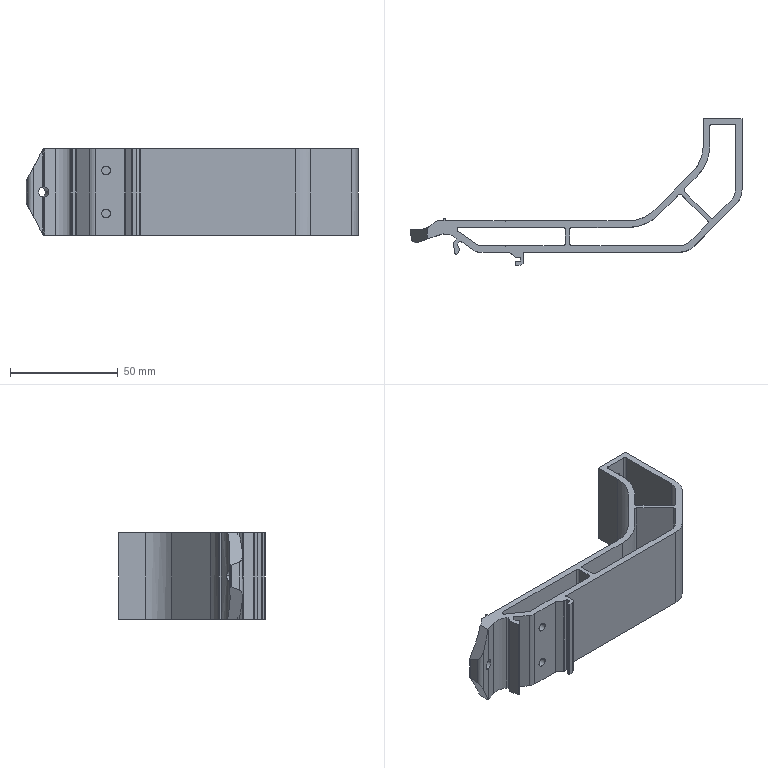Part | STEP file | 51E-01213JG10 | 1 solid | 123 faces | box 154.2 x 68 x 40 mm | volume 48152 mm3 | cylinder 62 | plane 61 | commonest cylinder face diameters 0.6 x20 2 x15 4 x6 6.5 x4 0.4 x2 1 x2